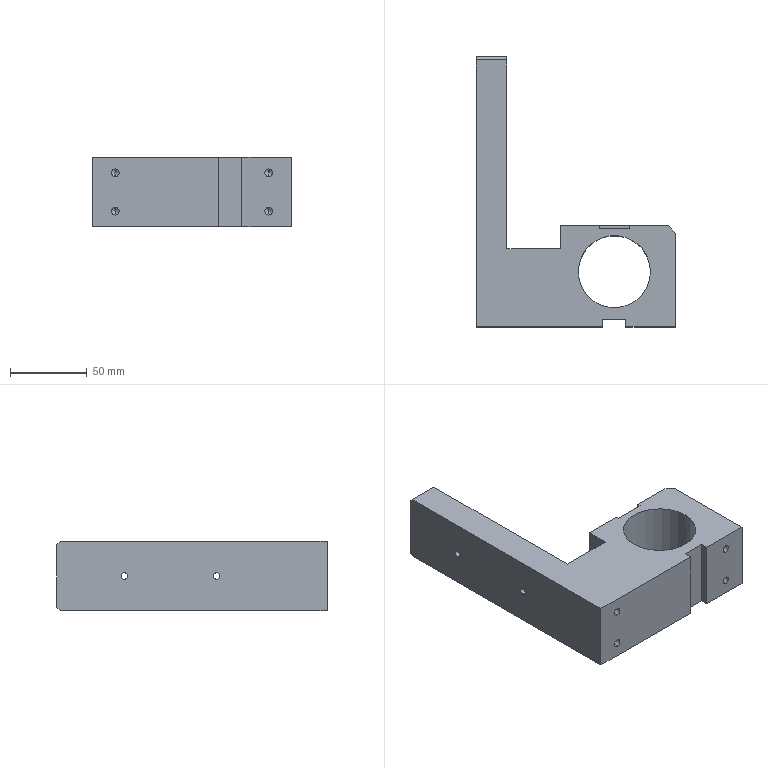Part | SolidWorks | features HoleWzd 4, Chamfer 2, ICE 2, Extrusion 1 | 1 solid | 67 faces | box 130 x 176 x 45 mm | volume 376408 mm3 | cylinder 26 | plane 21 | cone 20 | commonest cylinder face diameters 5 x12 3.3 x8 4.2 x4 47 x2